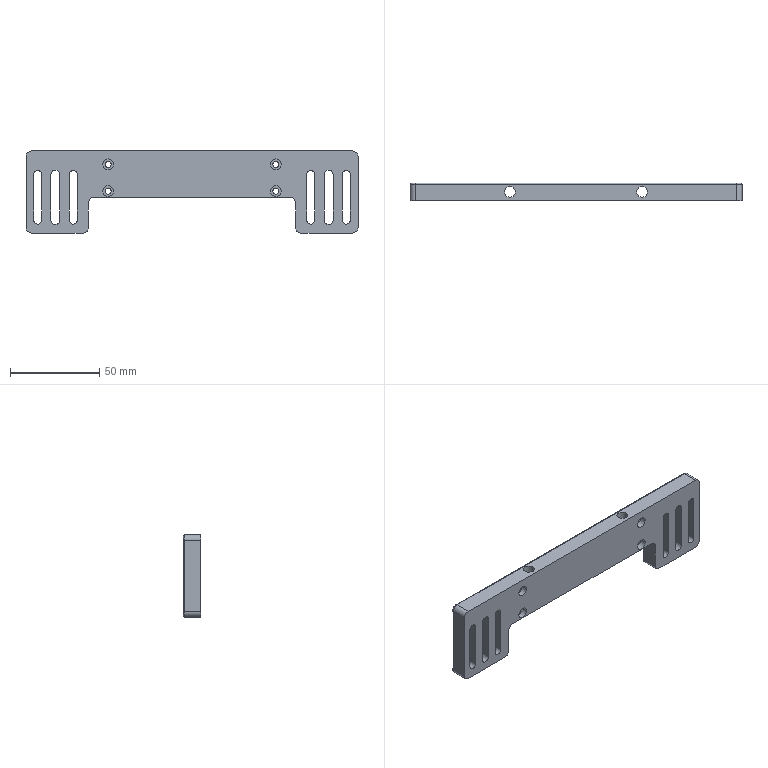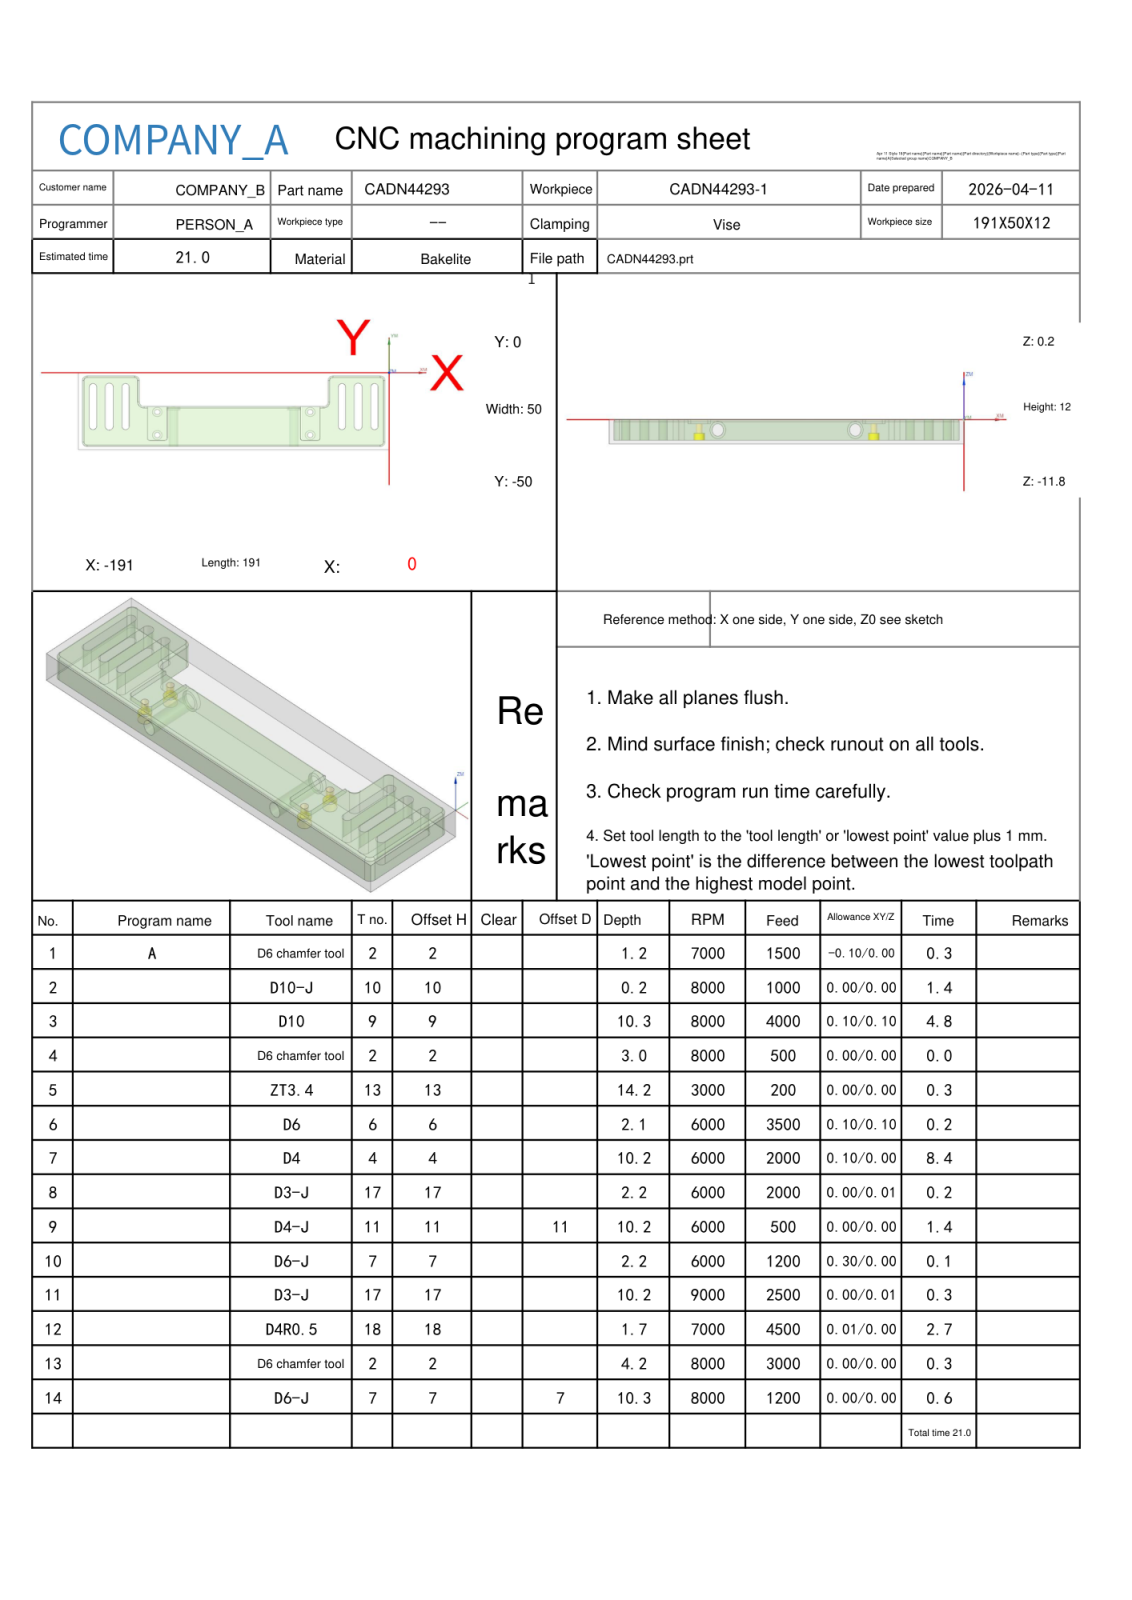NC program | NX | posted by the shop | part box 186 x 10 x 46 mm
Lines 1 to 1587 of 7485:
%
O0001
(Machine time: 23.98 MIN)
(===Total Tool:10===)
(T2=D6 chamfer tool   D=6.   R=0.   D-  H02 Z=-4.   )
(T10=D10-J  D=10.  R=0.   D-  H10 Z=-0.   )
(T9=D10     D=10.  R=0.   D-  H09 Z=-10.1 )
(T13=ZT3.4  D=3.4  DR_a=118 D-  H13 Z=-14.  )
(T6=D6      D=6.   R=0.   D-  H06 Z=-1.9  )
(T4=D4      D=4.   R=0.   D-  H04 Z=-10.  )
(T17=D3-J   D=3.   R=0.   D-  H17 Z=-9.95 )
(T11=D4-J   D=4.   R=0.   D11 H11 Z=-10.  )
(T7=D6-J    D=6.   R=0.   D-  H07 Z=-10.1 )
(T18=D4R0.5 D=4.   R=0.5  D-  H18 Z=-1.5  )
G80 G90 G17 G49 G40
G91 G28 Z0
M01
N1 T02 M06
(D6 chamfer tool  D=6. R=0. H=02 ce=-0.10 di=0.00)
G00 G90 G54 X-152.6 Y-14.634 M03 S7000
G43 H02 Z20.
M08
Z2.5
G01 Y-19.112 Z.87 F1500.
X-152.561 Y-19.417 Z.758
X-152.478 Y-19.714 Z.646
X-152.353 Y-19.995 Z.534
X-152.188 Y-20.254 Z.422
X-151.987 Y-20.487 Z.31
X-151.754 Y-20.688 Z.198
X-151.495 Y-20.853 Z.086
X-151.214 Y-20.978 Z-.025
X-150.917 Y-21.061 Z-.137
X-150.612 Y-21.1 Z-.249
X-148.55 Z-1.
X-40.5
G03 X-38.4 Y-19. I0.0 J2.1
G01 Y-5.
G02 X-34.5 Y-1.1 I3.9 J0.0
G01 X-5.5
G02 X-1.6 Y-5. I0.0 J-3.9
G01 Y-45.
G02 X-5.5 Y-48.9 I-3.9 J0.0
G01 X-185.5
G02 X-189.4 Y-45. I0.0 J3.9
G01 Y-5.
G02 X-185.5 Y-1.1 I3.9 J0.0
G01 X-156.5
G02 X-152.6 Y-5. I0.0 J-3.9
G01 Y-19.
G03 X-150.5 Y-21.1 I2.1 J0.0
G01 X-148.55
X-148.05
Z1.5
G00 Z20.
G91 G28 Z0.0
M05
M09
G91 G28 Z0.0
M01
N2 T10 M06
(D10-J  D=10. R=0. H=10 ce=0.00 di=0.00)
G00 G90 G54 X14.499 Y-44.782 M03 S8000
G43 H10 Z20.
M08
Z2.
G01 Z0.0 F1000.
X2.499 Y-44.912
X-192.413 Y-47.027
X-192.423
G02 X-193.412 Y-46.175 I0.0 J1.
X-193.499 Y-45. I7.912 J1.175
G01 Y-41.202
G02 X-192.511 Y-40.203 I1. J-.001
G01 X1.511 Y-38.098
G03 X2.499 Y-37.099 I-.012 J1.
G01 Y-32.172
G03 X1.599 Y-31.272 I-.9 J0.0
G01 X1.589
X-192.59 Y-33.379
X-192.599
G02 X-193.499 Y-32.48 I0.0 J.9
G01 Y-27.553
G02 X-192.51 Y-26.553 I1. J0.0
G01 X1.511 Y-24.447
G03 X2.499 Y-23.448 I-.012 J1.
G01 Y-18.521
G03 X1.599 Y-17.621 I-.9 J0.0
G01 X1.589
X-192.59 Y-19.728
X-192.599
G02 X-193.499 Y-18.829 I0.0 J.9
G01 Y-13.902
G02 X-192.51 Y-12.902 I1. J0.0
G01 X1.511 Y-10.797
G03 X2.499 Y-9.798 I-.012 J1.
G01 Y-5.
X2.498 Y-4.854
G03 X1.598 Y-3.971 I-.9 J-.017
G01 X1.589
X-193.499 Y-6.088
X-205.499 Y-6.218
Z2.
G00 Z20.
G91 G28 Z0.0
M05
M09
G91 G28 Z0.0
M01
N3 T09 M06
(D10  D=10. R=0. H=09 ce=0.10 di=0.10)
G00 G90 G54 X-62.968 Y12. M03 S8000
G43 H09 Z10.2
M08
Z.719
G01 Z-.481 F4000.
G02 X-61.259 Y7.416 I-5.291 J-4.584
X-61.689 Y5. I-7. J0.0
G03 X-61.821 Y4.634 I27.189 J-10.
G02 X-62.76 Y3.97 I-.942 J.336
G01 X-128.24
G02 X-129.112 Y4.485 I.003 J1.
G03 X-129.986 Y5. I-.874 J-.485
G01 X-135.981
G03 X-136.581 Y4.4 I0.0 J-.6
X-136.526 Y4.15 I.6 J0.0
G02 X-134.714 Y-2.162 I-19.974 J-9.15
G03 X-133.725 Y-3.03 I.991 J.132
G01 X-57.275
G03 X-56.286 Y-2.162 I-.002 J1.
G02 X-54.343 Y4.429 I21.786 J-2.838
X-53.441 Y5. I.903 J-.429
G01 X-46.503
G02 X-46.103 Y4.6 I0.0 J-.4
X-46.191 Y4.35 I-.4 J0.0
G03 X-49.47 Y-5. I11.691 J-9.35
G01 Y-9.685
G02 X-50.47 Y-10.684 I-1. J.001
X-50.78 Y-10.634 I0.0 J1.
G03 X-54.545 Y-10.03 I-3.777 J-11.503
G01 X-136.483
G03 X-140.217 Y-10.645 I.082 J-12.149
G02 X-140.53 Y-10.695 I-.313 J.95
X-141.53 Y-9.696 I0.0 J1.
G01 Y-5.
G03 X-144.743 Y4.267 I-14.97 J0.0
X-145.45 Y4.61 I-.707 J-.557
X-146.051 Y4.38 I0.0 J-.9
G01 X-149.867 Y.954
G03 X-150.199 Y.21 I.668 J-.744
X-150.013 Y-.37 I1. J0.0
G02 X-148.53 Y-5. I-6.487 J-4.63
G01 Y-17.035
G02 X-143.45 Y-22.148 I-.033 J-5.113
G01 Y-22.186
Y-38.9
X-141.55
Y-22.227
Y-22.179
G02 X-136.45 Y-17.03 I5.149 J0.0
G01 X-54.55
G02 X-49.45 Y-22.137 I-.007 J-5.107
G01 Y-22.144
Y-38.9
X-47.55
Y-22.144
G02 X-42.47 Y-17.034 I5.116 J-.006
G01 Y-5.
G02 X-34.5 Y2.97 I7.97 J0.0
G01 X-5.5
G02 X2.47 Y-5. I0.0 J-7.97
G01 Y-45.
G02 X-5.5 Y-52.97 I-7.97 J0.0
G01 X-185.5
G02 X-193.47 Y-45. I0.0 J7.97
G01 Y-5.
G02 X-185.5 Y2.97 I7.97 J0.0
G01 X-156.5
G02 X-148.573 Y-4.171 I0.0 J-7.97
X-148.537 Y-4.67 I-7.927 J-.829
G03 X-141.543 Y-11.38 I6.994 J.29
X-141.253 Y-11.374 I0.0 J7.
G01 Z.719
G00 Z3.
G01 X-63.12 Y12. F6000.
G00 Z.238
G01 Z-.962 F4000.
G02 X-61.401 Y7.406 I-5.281 J-4.594
X-61.827 Y5. I-7. J0.0
G03 X-61.914 Y4.761 I27.327 J-10.
G02 X-62.851 Y4.099 I-.941 J.339
G01 X-128.149
G02 X-128.981 Y4.55 I.004 J1.
G03 X-129.816 Y5. I-.835 J-.55
G01 X-135.839
G03 X-136.438 Y4.4 I0.0 J-.6
X-136.385 Y4.152 I.6 J0.0
G02 X-134.6 Y-2.038 I-20.115 J-9.152
G03 X-133.612 Y-2.901 I.991 J.137
G01 X-57.388
G03 X-56.4 Y-2.038 I-.003 J1.
G02 X-54.488 Y4.427 I21.9 J-2.962
X-53.584 Y5. I.904 J-.427
G01 X-46.668
G02 X-46.268 Y4.6 I0.0 J-.4
X-46.354 Y4.352 I-.4 J0.0
G03 X-49.599 Y-5. I11.854 J-9.352
G01 Y-9.513
G02 X-50.599 Y-10.511 I-1. J.002
X-50.899 Y-10.465 I0.0 J1.
G03 X-54.549 Y-9.901 I-3.652 J-11.537
G01 X-136.451
G03 X-140.101 Y-10.465 I.002 J-12.101
G02 X-140.401 Y-10.511 I-.3 J.954
X-141.401 Y-9.513 I0.0 J1.
G01 Y-5.
G03 X-144.576 Y4.263 I-15.099 J0.0
X-145.286 Y4.611 I-.711 J-.552
X-145.882 Y4.385 I0.0 J-.9
G01 X-149.724 Y.99
G03 X-150.061 Y.241 I.663 J-.749
X-149.879 Y-.335 I1. J0.0
G02 X-148.401 Y-5. I-6.621 J-4.665
G01 Y-16.903
G02 X-143.447 Y-22.008 I-.154 J-5.106
G01 X-143.45 Y-22.186
Y-38.9
X-141.55
Y-22.002
G02 X-136.45 Y-16.901 I5.101 J0.0
G01 X-54.55
G02 X-49.45 Y-22.001 I-.001 J-5.101
G01 Y-38.9
X-47.55
Y-22.002
G02 X-42.599 Y-16.904 I5.102 J-.001
G01 Y-5.
G02 X-34.5 Y3.099 I8.099 J0.0
G01 X-5.5
G02 X2.599 Y-5. I0.0 J-8.099
G01 Y-45.
G02 X-5.5 Y-53.099 I-8.099 J0.0
G01 X-185.5
G02 X-193.599 Y-45. I0.0 J8.099
G01 Y-5.
G02 X-185.5 Y3.099 I8.099 J0.0
G01 X-156.5
G02 X-148.447 Y-4.139 I0.0 J-8.099
X-148.409 Y-4.637 I-8.053 J-.861
G03 X-141.416 Y-11.324 I6.993 J.313
X-141.102 Y-11.317 I0.0 J7.
G01 Z.238
G00 Z2.519
G01 X-63.12 Y12. F6000.
G00 Z-.243
G01 Z-1.443 F4000.
G02 X-61.402 Y7.405 I-5.281 J-4.595
X-61.828 Y5. I-7. J0.0
G03 X-61.914 Y4.761 I27.328 J-10.
G02 X-62.851 Y4.1 I-.941 J.339
G01 X-128.149
G02 X-128.981 Y4.55 I.004 J1.
G03 X-129.815 Y5. I-.835 J-.55
G01 X-135.838
G03 X-136.438 Y4.4 I0.0 J-.6
X-136.384 Y4.152 I.6 J0.0
G02 X-134.599 Y-2.038 I-20.116 J-9.152
G03 X-133.612 Y-2.901 I.991 J.137
G01 X-131.103 Y-2.9
X-59.857 Y-2.901
X-57.388
G03 X-56.401 Y-2.038 I-.003 J1.
G02 X-54.489 Y4.427 I21.901 J-2.962
X-53.585 Y5. I.904 J-.427
G01 X-46.669
G02 X-46.269 Y4.6 I0.0 J-.4
X-46.355 Y4.352 I-.4 J0.0
G03 X-49.6 Y-5. I11.855 J-9.352
G01 Y-9.512
G02 X-50.6 Y-10.51 I-1. J.002
X-50.899 Y-10.464 I0.0 J1.
G03 X-54.55 Y-9.9 I-3.651 J-11.536
G01 X-57.054
X-57.202 Y-9.901
X-57.388
X-59.96 Y-9.9
X-131.072 Y-9.901
X-133.798
X-133.946 Y-9.9
X-136.476
G03 X-140.101 Y-10.464 I.026 J-12.1
G02 X-140.4 Y-10.51 I-.299 J.954
X-141.4 Y-9.512 I0.0 J1.
G01 Y-5.
G03 X-144.575 Y4.263 I-15.1 J0.0
X-145.286 Y4.611 I-.711 J-.552
X-145.881 Y4.385 I0.0 J-.9
G01 X-149.723 Y.99
G03 X-150.061 Y.241 I.663 J-.749
X-149.878 Y-.335 I1. J0.0
G02 X-148.4 Y-5. I-6.622 J-4.665
G01 Y-16.902
G02 X-143.45 Y-22. I-.15 J-5.098
G01 Y-38.9
X-141.55
Y-22.
G02 X-136.45 Y-16.9 I5.1 J0.0
G01 X-133.962
X-133.814 Y-16.901
X-130.971 Y-16.9
X-59.996 Y-16.901
X-57.186
X-57.038 Y-16.9
X-54.55
G02 X-49.45 Y-22. I0.0 J-5.1
G01 Y-38.9
X-47.55
Y-22.
G02 X-42.6 Y-16.902 I5.1 J0.0
G01 Y-5.
G02 X-34.5 Y3.1 I8.1 J0.0
G01 X-5.5
G02 X2.6 Y-5. I0.0 J-8.1
G01 Y-45.
G02 X-5.5 Y-53.1 I-8.1 J0.0
G01 X-185.5
G02 X-193.6 Y-45. I0.0 J8.1
G01 Y-5.
G02 X-185.5 Y3.1 I8.1 J0.0
G01 X-156.5
G02 X-148.446 Y-4.139 I0.0 J-8.1
X-148.408 Y-4.637 I-8.054 J-.861
G03 X-141.415 Y-11.324 I6.993 J.314
X-141.102 Y-11.317 I0.0 J7.
G01 Z-.243
G00 Z2.038
G01 X-63.12 Y12. F6000.
G00 Z-.724
G01 Z-1.924 F4000.
G02 X-61.402 Y7.406 I-5.281 J-4.594
X-61.828 Y5. I-7. J0.0
G03 X-61.914 Y4.761 I27.328 J-10.
G02 X-62.851 Y4.1 I-.941 J.339
G01 X-128.149
G02 X-128.981 Y4.55 I.004 J1.
G03 X-129.815 Y5. I-.835 J-.55
G01 X-135.838
G03 X-136.438 Y4.4 I0.0 J-.6
X-136.384 Y4.152 I.6 J0.0
G02 X-134.599 Y-2.038 I-20.116 J-9.152
G03 X-133.612 Y-2.901 I.991 J.137
G01 X-131.097 Y-2.9
X-59.861 Y-2.901
X-57.388
G03 X-56.401 Y-2.038 I-.003 J1.
G02 X-54.489 Y4.427 I21.901 J-2.962
X-53.585 Y5. I.904 J-.427
G01 X-46.669
G02 X-46.269 Y4.6 I0.0 J-.4
X-46.355 Y4.352 I-.4 J0.0
G03 X-49.6 Y-5. I11.855 J-9.352
G01 Y-8.938
G02 X-50.597 Y-9.935 I-1. J.003
G01 X-53.627
G03 X-54.55 Y-9.9 I-.923 J-12.065
G01 X-57.053
X-57.211 Y-9.901
X-57.388
X-59.963 Y-9.9
X-131.07 Y-9.901
X-133.789
X-133.947 Y-9.9
X-136.761
X-136.869 Y-9.907
G03 X-137.373 Y-9.935 I.419 J-12.093
G01 X-140.403
G02 X-141.4 Y-8.938 I.003 J1.
G01 Y-5.
G03 X-144.575 Y4.263 I-15.1 J0.0
X-145.286 Y4.611 I-.711 J-.552
X-145.881 Y4.385 I0.0 J-.9
G01 X-149.723 Y.99
G03 X-150.061 Y.241 I.663 J-.749
X-149.878 Y-.335 I1. J0.0
G02 X-148.4 Y-5. I-6.622 J-4.665
G01 Y-16.902
G02 X-147.952 Y-16.935 I-.15 J-5.098
G01 X-137.048
G02 X-136.526 Y-16.9 I.604 J-5.065
G01 X-133.962
X-133.803 Y-16.901
X-130.971 Y-16.9
X-59.995 Y-16.901
X-57.197
X-57.038 Y-16.9
X-54.55
G02 X-53.952 Y-16.935 I0.0 J-5.1
G01 X-43.048
G02 X-42.6 Y-16.902 I.598 J-5.065
G01 Y-5.
G02 X-34.5 Y3.1 I8.1 J0.0
G01 X-5.5
G02 X2.6 Y-5. I0.0 J-8.1
G01 Y-45.
G02 X-5.5 Y-53.1 I-8.1 J0.0
G01 X-185.5
G02 X-193.6 Y-45. I0.0 J8.1
G01 Y-5.
G02 X-185.5 Y3.1 I8.1 J0.0
G01 X-156.5
G02 X-148.446 Y-4.139 I0.0 J-8.1
X-148.408 Y-4.637 I-8.054 J-.861
G03 X-141.415 Y-11.324 I6.993 J.314
X-141.102 Y-11.317 I0.0 J7.
G01 Z-.724
G00 Z1.557
G01 X-63.12 Y12. F6000.
G00 Z-1.205
G01 Z-2.405 F4000.
G02 X-61.402 Y7.405 I-5.281 J-4.595
X-61.828 Y5. I-7. J0.0
G03 X-61.914 Y4.76 I27.328 J-10.
G02 X-62.851 Y4.1 I-.941 J.34
G01 X-128.149
G02 X-128.981 Y4.55 I.004 J1.
G03 X-129.815 Y5. I-.835 J-.55
G01 X-135.838
G03 X-136.438 Y4.4 I0.0 J-.6
X-136.384 Y4.152 I.6 J0.0
G02 X-134.599 Y-2.038 I-20.116 J-9.152
G03 X-133.613 Y-2.901 I.99 J.138
G01 X-131.092 Y-2.9
X-59.861 Y-2.901
X-57.387
G03 X-56.401 Y-2.038 I-.004 J1.
G02 X-54.489 Y4.427 I21.901 J-2.962
X-53.585 Y5. I.904 J-.427
G01 X-46.669
G02 X-46.269 Y4.6 I0.0 J-.4
X-46.355 Y4.352 I-.4 J0.0
G03 X-49.6 Y-5. I11.855 J-9.352
G01 Y-8.903
G02 X-50.597 Y-9.9 I-1. J.003
G01 X-57.052
X-57.222 Y-9.901
X-57.387
X-59.963 Y-9.9
X-131.069 Y-9.901
X-133.778
X-133.948 Y-9.9
X-140.403
G02 X-141.4 Y-8.903 I.003 J1.
G01 Y-5.
G03 X-144.575 Y4.263 I-15.1 J0.0
X-145.286 Y4.611 I-.711 J-.552
X-145.881 Y4.385 I0.0 J-.9
G01 X-149.723 Y.99
G03 X-150.061 Y.241 I.663 J-.749
X-149.878 Y-.335 I1. J0.0
G02 X-148.4 Y-5. I-6.622 J-4.665
G01 Y-16.9
X-133.962
X-133.792 Y-16.901
X-130.971 Y-16.9
X-59.995 Y-16.901
X-57.208
X-57.038 Y-16.9
X-42.6
Y-5.
G02 X-34.5 Y3.1 I8.1 J0.0
G01 X-5.5
G02 X2.6 Y-5. I0.0 J-8.1
G01 Y-45.
G02 X-5.5 Y-53.1 I-8.1 J0.0
G01 X-185.5
G02 X-193.6 Y-45. I0.0 J8.1
G01 Y-5.
G02 X-185.5 Y3.1 I8.1 J0.0
G01 X-156.5
G02 X-148.446 Y-4.139 I0.0 J-8.1
X-148.408 Y-4.637 I-8.054 J-.861
G03 X-141.415 Y-11.324 I6.993 J.314
X-141.102 Y-11.317 I0.0 J7.
G01 Z-1.205
G00 Z1.076
G01 X-63.12 Y12. F6000.
G00 Z-1.686
G01 Z-2.886 F4000.
G02 X-61.402 Y7.406 I-5.281 J-4.595
X-61.828 Y5. I-7. J0.0
G03 X-61.914 Y4.76 I27.328 J-10.
G02 X-62.85 Y4.1 I-.941 J.34
G01 X-128.15
G02 X-128.981 Y4.55 I.004 J1.
G03 X-129.815 Y5. I-.835 J-.55
G01 X-135.838
G03 X-136.438 Y4.4 I0.0 J-.6
X-136.384 Y4.152 I.6 J0.0
G02 X-134.599 Y-2.039 I-20.116 J-9.152
G03 X-133.613 Y-2.901 I.99 J.138
G01 X-131.086 Y-2.9
X-59.865 Y-2.901
X-57.387
G03 X-56.401 Y-2.039 I-.004 J1.
G02 X-54.489 Y4.427 I21.901 J-2.961
X-53.585 Y5. I.904 J-.427
G01 X-46.669
G02 X-46.269 Y4.6 I0.0 J-.4
X-46.355 Y4.352 I-.4 J0.0
G03 X-49.6 Y-5. I11.855 J-9.352
G01 Y-8.903
G02 X-50.597 Y-9.9 I-1. J.003
G01 X-57.051
X-57.234 Y-9.901
X-57.387
X-59.965 Y-9.9
X-131.068 Y-9.901
X-133.766
X-133.949 Y-9.9
X-140.403
G02 X-141.4 Y-8.903 I.003 J1.
G01 Y-5.
G03 X-144.575 Y4.263 I-15.1 J0.0
X-145.286 Y4.611 I-.711 J-.552
X-145.881 Y4.385 I0.0 J-.9
G01 X-149.723 Y.99
G03 X-150.061 Y.241 I.663 J-.749
X-149.878 Y-.335 I1. J0.0
G02 X-148.4 Y-5. I-6.622 J-4.665
G01 Y-16.9
X-133.962
X-133.779 Y-16.901
X-130.971 Y-16.9
X-59.993 Y-16.901
X-57.221
X-57.038 Y-16.9
X-42.6
Y-5.
G02 X-34.5 Y3.1 I8.1 J0.0
G01 X-5.5
G02 X2.6 Y-5. I0.0 J-8.1
G01 Y-45.
G02 X-5.5 Y-53.1 I-8.1 J0.0
G01 X-185.5
G02 X-193.6 Y-45. I0.0 J8.1
G01 Y-5.
G02 X-185.5 Y3.1 I8.1 J0.0
G01 X-156.5
G02 X-148.446 Y-4.139 I0.0 J-8.1
X-148.408 Y-4.637 I-8.054 J-.861
G03 X-141.415 Y-11.324 I6.993 J.314
X-141.102 Y-11.317 I0.0 J7.
G01 Z-1.686
G00 Z.595
G01 X-63.12 Y12. F6000.
G00 Z-2.167
G01 Z-3.367 F4000.
G02 X-61.402 Y7.406 I-5.281 J-4.594
X-61.828 Y5. I-7. J0.0
G03 X-61.914 Y4.76 I27.328 J-10.
G02 X-62.85 Y4.1 I-.94 J.34
G01 X-128.15
G02 X-128.981 Y4.55 I.005 J1.
G03 X-129.815 Y5. I-.835 J-.55
G01 X-135.838
G03 X-136.438 Y4.4 I0.0 J-.6
X-136.384 Y4.152 I.6 J0.0
G02 X-134.599 Y-2.039 I-20.116 J-9.152
G03 X-133.613 Y-2.901 I.99 J.138
G01 X-131.083 Y-2.9
X-59.865 Y-2.901
X-57.387
G03 X-56.401 Y-2.039 I-.004 J1.
G02 X-54.489 Y4.427 I21.901 J-2.961
X-53.585 Y5. I.904 J-.427
G01 X-46.669
G02 X-46.269 Y4.6 I0.0 J-.4
X-46.355 Y4.352 I-.4 J0.0
G03 X-49.6 Y-5. I11.855 J-9.352
G01 Y-8.904
G02 X-50.596 Y-9.9 I-1. J.004
G01 X-57.05
X-57.249 Y-9.901
X-57.387
X-59.965 Y-9.9
X-131.068 Y-9.901
X-133.751
X-133.95 Y-9.9
X-140.404
G02 X-141.4 Y-8.904 I.004 J1.
G01 Y-5.
G03 X-144.575 Y4.263 I-15.1 J0.0
X-145.286 Y4.611 I-.711 J-.552
X-145.881 Y4.385 I0.0 J-.9
G01 X-149.723 Y.99
G03 X-150.061 Y.241 I.663 J-.749
X-149.878 Y-.335 I1. J0.0
G02 X-148.4 Y-5. I-6.622 J-4.665
G01 Y-16.9
X-133.962
X-133.763 Y-16.901
X-130.971 Y-16.9
X-59.993 Y-16.901
X-57.237
X-57.038 Y-16.9
X-42.6
Y-5.
G02 X-34.5 Y3.1 I8.1 J0.0
G01 X-5.5
G02 X2.6 Y-5. I0.0 J-8.1
G01 Y-45.
G02 X-5.5 Y-53.1 I-8.1 J0.0
G01 X-185.5
G02 X-193.6 Y-45. I0.0 J8.1
G01 Y-5.
G02 X-185.5 Y3.1 I8.1 J0.0
G01 X-156.5
G02 X-148.446 Y-4.139 I0.0 J-8.1
X-148.408 Y-4.637 I-8.054 J-.861
G03 X-141.415 Y-11.324 I6.993 J.314
X-141.102 Y-11.317 I0.0 J7.
G01 Z-2.167
G00 Z.114
G01 X-63.12 Y12. F6000.
G00 Z-2.648
G01 Z-3.848 F4000.
G02 X-61.402 Y7.406 I-5.281 J-4.595
X-61.828 Y5. I-7. J0.0
G03 X-61.914 Y4.76 I27.328 J-10.
G02 X-62.85 Y4.1 I-.94 J.34
G01 X-128.15
G02 X-128.981 Y4.55 I.005 J1.
G03 X-129.815 Y5. I-.835 J-.55
G01 X-135.838
G03 X-136.438 Y4.4 I0.0 J-.6
X-136.384 Y4.152 I.6 J0.0
G02 X-134.599 Y-2.039 I-20.116 J-9.152
G03 X-133.613 Y-2.901 I.99 J.138
G01 X-131.083 Y-2.9
X-59.867 Y-2.901
X-57.387
G03 X-56.401 Y-2.039 I-.004 J1.
G02 X-54.489 Y4.427 I21.901 J-2.961
X-53.585 Y5. I.904 J-.427
G01 X-46.669
G02 X-46.269 Y4.6 I0.0 J-.4
X-46.355 Y4.352 I-.4 J0.0
G03 X-49.6 Y-5. I11.855 J-9.352
G01 Y-8.904
G02 X-50.596 Y-9.9 I-1. J.004
G01 X-57.049
X-57.266 Y-9.901
X-57.387
X-59.967 Y-9.9
X-131.068 Y-9.901
X-133.734
X-133.951 Y-9.9
X-140.404
G02 X-141.4 Y-8.904 I.004 J1.
G01 Y-5.
G03 X-144.575 Y4.263 I-15.1 J0.0
X-145.286 Y4.611 I-.711 J-.552
X-145.881 Y4.385 I0.0 J-.9
G01 X-149.723 Y.99
G03 X-150.061 Y.241 I.663 J-.749
X-149.878 Y-.335 I1. J0.0
G02 X-148.4 Y-5. I-6.622 J-4.665
G01 Y-16.9
X-133.962
X-133.745 Y-16.901
X-130.971 Y-16.9
X-59.992 Y-16.901
X-57.255
X-57.038 Y-16.9
X-42.6
Y-5.
G02 X-34.5 Y3.1 I8.1 J0.0
G01 X-5.5
G02 X2.6 Y-5. I0.0 J-8.1
G01 Y-45.
G02 X-5.5 Y-53.1 I-8.1 J0.0
G01 X-185.5
G02 X-193.6 Y-45. I0.0 J8.1
G01 Y-5.
G02 X-185.5 Y3.1 I8.1 J0.0
G01 X-156.5
G02 X-148.446 Y-4.139 I0.0 J-8.1
X-148.408 Y-4.637 I-8.054 J-.861
G03 X-141.415 Y-11.324 I6.993 J.314
X-141.102 Y-11.317 I0.0 J7.
G01 Z-2.648
G00 Z-.367
G01 X-63.12 Y12. F6000.
G00 Z-3.129
G01 Z-4.329 F4000.
G02 X-61.402 Y7.406 I-5.281 J-4.595
X-61.828 Y5. I-7. J0.0
G03 X-61.914 Y4.762 I27.328 J-10.
G02 X-62.852 Y4.1 I-.941 J.338
G01 X-128.148
G02 X-128.981 Y4.55 I.003 J1.
G03 X-129.815 Y5. I-.835 J-.55
G01 X-135.838
G03 X-136.438 Y4.4 I0.0 J-.6
X-136.384 Y4.152 I.6 J0.0
G02 X-134.6 Y-2.036 I-20.116 J-9.152
G03 X-133.611 Y-2.9 I.991 J.136
G01 X-57.389
G03 X-56.4 Y-2.036 I-.002 J1.
G02 X-54.489 Y4.427 I21.9 J-2.964
X-53.585 Y5. I.904 J-.427
G01 X-46.669
G02 X-46.269 Y4.6 I0.0 J-.4
X-46.355 Y4.352 I-.4 J0.0
G03 X-49.6 Y-5. I11.855 J-9.352
G01 Y-8.901
G02 X-50.599 Y-9.9 I-1. J.001
G01 X-140.401
G02 X-141.4 Y-8.901 I.001 J1.
G01 Y-5.
G03 X-144.575 Y4.263 I-15.1 J0.0
X-145.286 Y4.611 I-.711 J-.552
X-145.881 Y4.385 I0.0 J-.9
G01 X-149.723 Y.99
G03 X-150.061 Y.241 I.663 J-.749
X-149.878 Y-.335 I1. J0.0
G02 X-148.4 Y-5. I-6.622 J-4.665
G01 Y-16.9
X-42.6
Y-5.
G02 X-34.5 Y3.1 I8.1 J0.0
G01 X-5.5
G02 X2.6 Y-5. I0.0 J-8.1
G01 Y-45.
G02 X-5.5 Y-53.1 I-8.1 J0.0
G01 X-185.5
G02 X-193.6 Y-45. I0.0 J8.1
G01 Y-5.
G02 X-185.5 Y3.1 I8.1 J0.0
G01 X-156.5
G02 X-148.446 Y-4.139 I0.0 J-8.1
X-148.408 Y-4.637 I-8.054 J-.861
G03 X-141.415 Y-11.324 I6.993 J.314
X-141.102 Y-11.317 I0.0 J7.
G01 Z-3.129
G00 Z-.848
G01 X-63.12 Y12. F6000.
G00 Z-3.61
G01 Z-4.81 F4000.
G02 X-61.402 Y7.405 I-5.281 J-4.595
X-61.828 Y5. I-7. J0.0
G03 X-61.914 Y4.761 I27.328 J-10.
G02 X-62.852 Y4.1 I-.941 J.339
G01 X-128.148
G02 X-128.981 Y4.55 I.003 J1.
G03 X-129.815 Y5. I-.835 J-.55
G01 X-135.838
G03 X-136.438 Y4.4 I0.0 J-.6
X-136.384 Y4.152 I.6 J0.0
G02 X-134.6 Y-2.037 I-20.116 J-9.152
G03 X-133.611 Y-2.9 I.991 J.137
G01 X-57.389
G03 X-56.4 Y-2.037 I-.002 J1.
G02 X-54.489 Y4.427 I21.9 J-2.963
X-53.585 Y5. I.904 J-.427
G01 X-46.669
G02 X-46.269 Y4.6 I0.0 J-.4
X-46.355 Y4.352 I-.4 J0.0
G03 X-49.6 Y-5. I11.855 J-9.352
G01 Y-8.901
G02 X-50.599 Y-9.9 I-1. J.001
G01 X-140.401
G02 X-141.4 Y-8.901 I.001 J1.
G01 Y-5.
G03 X-144.575 Y4.263 I-15.1 J0.0
X-145.286 Y4.611 I-.711 J-.552
X-145.881 Y4.385 I0.0 J-.9
G01 X-149.723 Y.99
G03 X-150.061 Y.241 I.663 J-.749
X-149.878 Y-.335 I1. J0.0
G02 X-148.4 Y-5. I-6.622 J-4.665
G01 Y-16.9
X-42.6
Y-5.
G02 X-34.5 Y3.1 I8.1 J0.0
G01 X-5.5
G02 X2.6 Y-5. I0.0 J-8.1
G01 Y-45.
G02 X-5.5 Y-53.1 I-8.1 J0.0
G01 X-185.5
G02 X-193.6 Y-45. I0.0 J8.1
G01 Y-5.
G02 X-185.5 Y3.1 I8.1 J0.0
G01 X-156.5
G02 X-148.446 Y-4.139 I0.0 J-8.1
X-148.408 Y-4.637 I-8.054 J-.861
G03 X-141.415 Y-11.324 I6.993 J.314
X-141.102 Y-11.317 I0.0 J7.
G01 Z-3.61
G00 Z-1.329
G01 X-63.12 Y12. F6000.
G00 Z-4.09
G01 Z-5.29 F4000.
G02 X-61.402 Y7.406 I-5.281 J-4.595
X-61.828 Y5. I-7. J0.0
G03 X-61.914 Y4.762 I27.328 J-10.
G02 X-62.852 Y4.1 I-.941 J.338
G01 X-128.148
G02 X-128.981 Y4.55 I.003 J1.
G03 X-129.815 Y5. I-.835 J-.55
G01 X-135.838
G03 X-136.438 Y4.4 I0.0 J-.6
X-136.384 Y4.152 I.6 J0.0
G02 X-134.6 Y-2.036 I-20.116 J-9.152
G03 X-133.611 Y-2.9 I.991 J.136
G01 X-57.389
G03 X-56.4 Y-2.036 I-.002 J1.
G02 X-54.489 Y4.427 I21.9 J-2.964
X-53.585 Y5. I.904 J-.427
G01 X-46.669
G02 X-46.269 Y4.6 I0.0 J-.4
X-46.355 Y4.352 I-.4 J0.0
G03 X-49.6 Y-5. I11.855 J-9.352
G01 Y-8.901
G02 X-50.599 Y-9.9 I-1. J.001
G01 X-140.401
G02 X-141.4 Y-8.901 I.001 J1.
G01 Y-5.
G03 X-144.575 Y4.263 I-15.1 J0.0
X-145.286 Y4.611 I-.711 J-.552
X-145.881 Y4.385 I0.0 J-.9
G01 X-149.723 Y.99
G03 X-150.061 Y.241 I.663 J-.749
X-149.878 Y-.335 I1. J0.0
G02 X-148.4 Y-5. I-6.622 J-4.665
G01 Y-16.9
X-42.6
Y-5.
G02 X-34.5 Y3.1 I8.1 J0.0
G01 X-5.5
G02 X2.6 Y-5. I0.0 J-8.1
G01 Y-45.
G02 X-5.5 Y-53.1 I-8.1 J0.0
G01 X-185.5
G02 X-193.6 Y-45. I0.0 J8.1
G01 Y-5.
G02 X-185.5 Y3.1 I8.1 J0.0
G01 X-156.5
G02 X-148.446 Y-4.139 I0.0 J-8.1
X-148.408 Y-4.637 I-8.054 J-.861
G03 X-141.415 Y-11.324 I6.993 J.314
X-141.102 Y-11.317 I0.0 J7.
G01 Z-4.09
G00 Z-1.81
G01 X-63.12 Y12. F6000.
G00 Z-4.571
G01 Z-5.771 F4000.
G02 X-61.402 Y7.405 I-5.281 J-4.595
X-61.828 Y5. I-7. J0.0
G03 X-61.914 Y4.761 I27.328 J-10.
G02 X-62.852 Y4.1 I-.941 J.339
G01 X-128.148
G02 X-128.981 Y4.55 I.003 J1.
G03 X-129.815 Y5. I-.835 J-.55
G01 X-135.838
G03 X-136.438 Y4.4 I0.0 J-.6
X-136.384 Y4.152 I.6 J0.0
G02 X-134.6 Y-2.037 I-20.116 J-9.152
G03 X-133.611 Y-2.9 I.991 J.137
G01 X-57.389
G03 X-56.4 Y-2.037 I-.002 J1.
G02 X-54.489 Y4.427 I21.9 J-2.963
X-53.585 Y5. I.904 J-.427
G01 X-46.669
G02 X-46.269 Y4.6 I0.0 J-.4
X-46.355 Y4.352 I-.4 J0.0
G03 X-49.6 Y-5. I11.855 J-9.352
G01 Y-8.901
G02 X-50.599 Y-9.9 I-1. J.001
G01 X-140.401
G02 X-141.4 Y-8.901 I.001 J1.
G01 Y-5.
G03 X-144.575 Y4.263 I-15.1 J0.0
X-145.286 Y4.611 I-.711 J-.552
X-145.881 Y4.385 I0.0 J-.9
G01 X-149.723 Y.99
G03 X-150.061 Y.241 I.663 J-.749
X-149.878 Y-.335 I1. J0.0
G02 X-148.4 Y-5. I-6.622 J-4.665
G01 Y-16.9
X-42.6
Y-5.
G02 X-34.5 Y3.1 I8.1 J0.0
G01 X-5.5
G02 X2.6 Y-5. I0.0 J-8.1
G01 Y-45.
G02 X-5.5 Y-53.1 I-8.1 J0.0
G01 X-185.5
G02 X-193.6 Y-45. I0.0 J8.1
G01 Y-5.
G02 X-185.5 Y3.1 I8.1 J0.0
G01 X-156.5
G02 X-148.446 Y-4.139 I0.0 J-8.1
X-148.408 Y-4.637 I-8.054 J-.861
G03 X-141.415 Y-11.324 I6.993 J.314
X-141.102 Y-11.317 I0.0 J7.
G01 Z-4.571
G00 Z-2.29
G01 X-63.12 Y12. F6000.
G00 Z-5.052
G01 Z-6.252 F4000.
G02 X-61.402 Y7.406 I-5.281 J-4.595
X-61.828 Y5. I-7. J0.0
G03 X-61.914 Y4.762 I27.328 J-10.
G02 X-62.852 Y4.1 I-.941 J.338
G01 X-128.148
G02 X-128.981 Y4.55 I.003 J1.
G03 X-129.815 Y5. I-.835 J-.55
G01 X-135.838
G03 X-136.438 Y4.4 I0.0 J-.6
X-136.384 Y4.152 I.6 J0.0
G02 X-134.6 Y-2.036 I-20.116 J-9.152
G03 X-133.611 Y-2.9 I.991 J.136
G01 X-57.389
G03 X-56.4 Y-2.036 I-.002 J1.
G02 X-54.489 Y4.427 I21.9 J-2.964
X-53.585 Y5. I.904 J-.427
G01 X-46.669
G02 X-46.269 Y4.6 I0.0 J-.4
X-46.355 Y4.352 I-.4 J0.0
G03 X-49.6 Y-5. I11.855 J-9.352
G01 Y-8.901
G02 X-50.599 Y-9.9 I-1. J.001
G01 X-140.401
G02 X-141.4 Y-8.901 I.001 J1.
G01 Y-5.
G03 X-144.575 Y4.263 I-15.1 J0.0
X-145.286 Y4.611 I-.711 J-.552
X-145.881 Y4.385 I0.0 J-.9
G01 X-149.723 Y.99
G03 X-150.061 Y.241 I.663 J-.749
X-149.878 Y-.335 I1. J0.0
G02 X-148.4 Y-5. I-6.622 J-4.665
G01 Y-16.9
X-42.6
Y-5.
G02 X-34.5 Y3.1 I8.1 J0.0
G01 X-5.5
G02 X2.6 Y-5. I0.0 J-8.1
G01 Y-45.
G02 X-5.5 Y-53.1 I-8.1 J0.0
G01 X-185.5
G02 X-193.6 Y-45. I0.0 J8.1
G01 Y-5.
G02 X-185.5 Y3.1 I8.1 J0.0
G01 X-156.5
G02 X-148.446 Y-4.139 I0.0 J-8.1
X-148.408 Y-4.637 I-8.054 J-.861
G03 X-141.415 Y-11.324 I6.993 J.314
X-141.102 Y-11.317 I0.0 J7.
G01 Z-5.052
G00 Z-2.771
G01 X-63.12 Y12. F6000.
G00 Z-5.533
G01 Z-6.733 F4000.
G02 X-61.402 Y7.405 I-5.281 J-4.595
X-61.828 Y5. I-7. J0.0
G03 X-61.914 Y4.761 I27.328 J-10.
G02 X-62.852 Y4.1 I-.941 J.339
G01 X-128.148
G02 X-128.981 Y4.55 I.003 J1.
G03 X-129.815 Y5. I-.835 J-.55
G01 X-135.838
G03 X-136.438 Y4.4 I0.0 J-.6
X-136.384 Y4.152 I.6 J0.0
G02 X-134.6 Y-2.037 I-20.116 J-9.152
G03 X-133.611 Y-2.9 I.991 J.137
G01 X-57.389
G03 X-56.4 Y-2.037 I-.002 J1.
G02 X-54.489 Y4.427 I21.9 J-2.963
X-53.585 Y5. I.904 J-.427
G01 X-46.669
G02 X-46.269 Y4.6 I0.0 J-.4
X-46.355 Y4.352 I-.4 J0.0
G03 X-49.6 Y-5. I11.855 J-9.352
G01 Y-8.901
G02 X-50.599 Y-9.9 I-1. J.001
G01 X-140.401
G02 X-141.4 Y-8.901 I.001 J1.
G01 Y-5.
G03 X-144.575 Y4.263 I-15.1 J0.0
X-145.286 Y4.611 I-.711 J-.552
X-145.881 Y4.385 I0.0 J-.9
G01 X-149.723 Y.99
G03 X-150.061 Y.241 I.663 J-.749
X-149.878 Y-.335 I1. J0.0
G02 X-148.4 Y-5. I-6.622 J-4.665
G01 Y-16.9
X-42.6
Y-5.
G02 X-34.5 Y3.1 I8.1 J0.0
G01 X-5.5
G02 X2.6 Y-5. I0.0 J-8.1
G01 Y-45.
G02 X-5.5 Y-53.1 I-8.1 J0.0
G01 X-185.5
G02 X-193.6 Y-45. I0.0 J8.1
G01 Y-5.
G02 X-185.5 Y3.1 I8.1 J0.0
G01 X-156.5
G02 X-148.446 Y-4.139 I0.0 J-8.1
X-148.408 Y-4.637 I-8.054 J-.861
G03 X-141.415 Y-11.324 I6.993 J.314
X-141.102 Y-11.317 I0.0 J7.
G01 Z-5.533
G00 Z-3.252
G01 X-63.12 Y12. F6000.
G00 Z-6.014
G01 Z-7.214 F4000.
G02 X-61.402 Y7.406 I-5.281 J-4.595
X-61.828 Y5. I-7. J0.0
G03 X-61.914 Y4.762 I27.328 J-10.
G02 X-62.852 Y4.1 I-.941 J.338
G01 X-128.148
G02 X-128.981 Y4.55 I.003 J1.
G03 X-129.815 Y5. I-.835 J-.55
G01 X-135.838
G03 X-136.438 Y4.4 I0.0 J-.6
X-136.384 Y4.152 I.6 J0.0
G02 X-134.6 Y-2.036 I-20.116 J-9.152
G03 X-133.611 Y-2.9 I.991 J.136
G01 X-57.389
G03 X-56.4 Y-2.036 I-.002 J1.
G02 X-54.489 Y4.427 I21.9 J-2.964
X-53.585 Y5. I.904 J-.427
G01 X-46.669
G02 X-46.269 Y4.6 I0.0 J-.4
X-46.355 Y4.352 I-.4 J0.0
G03 X-49.6 Y-5. I11.855 J-9.352
G01 Y-8.901
G02 X-50.599 Y-9.9 I-1. J.001
G01 X-140.401
G02 X-141.4 Y-8.901 I.001 J1.
G01 Y-5.
G03 X-144.575 Y4.263 I-15.1 J0.0
X-145.286 Y4.611 I-.711 J-.552
X-145.881 Y4.385 I0.0 J-.9
G01 X-149.723 Y.99
G03 X-150.061 Y.241 I.663 J-.749
X-149.878 Y-.335 I1. J0.0
G02 X-148.4 Y-5. I-6.622 J-4.665
G01 Y-16.9
X-42.6
Y-5.
G02 X-34.5 Y3.1 I8.1 J0.0
G01 X-5.5
G02 X2.6 Y-5. I0.0 J-8.1
G01 Y-45.
G02 X-5.5 Y-53.1 I-8.1 J0.0
G01 X-185.5
G02 X-193.6 Y-45. I0.0 J8.1
G01 Y-5.
G02 X-185.5 Y3.1 I8.1 J0.0
G01 X-156.5
G02 X-148.446 Y-4.139 I0.0 J-8.1
X-148.408 Y-4.637 I-8.054 J-.861
G03 X-141.415 Y-11.324 I6.993 J.314
X-141.102 Y-11.317 I0.0 J7.
G01 Z-6.014
G00 Z-3.733
G01 X-63.12 Y12. F6000.
G00 Z-6.495
G01 Z-7.695 F4000.
G02 X-61.402 Y7.405 I-5.281 J-4.595
X-61.828 Y5. I-7. J0.0
G03 X-61.914 Y4.761 I27.328 J-10.
G02 X-62.852 Y4.1 I-.941 J.339
G01 X-128.148
G02 X-128.981 Y4.55 I.003 J1.
G03 X-129.815 Y5. I-.835 J-.55
G01 X-135.838
G03 X-136.438 Y4.4 I0.0 J-.6
X-136.384 Y4.152 I.6 J0.0
G02 X-134.6 Y-2.037 I-20.116 J-9.152
G03 X-133.611 Y-2.9 I.991 J.137
G01 X-57.389
G03 X-56.4 Y-2.037 I-.002 J1.
G02 X-54.489 Y4.427 I21.9 J-2.963
X-53.585 Y5. I.904 J-.427
G01 X-46.669
G02 X-46.269 Y4.6 I0.0 J-.4
X-46.355 Y4.352 I-.4 J0.0
G03 X-49.6 Y-5. I11.855 J-9.352
G01 Y-8.901
G02 X-50.599 Y-9.9 I-1. J.001
G01 X-140.401
G02 X-141.4 Y-8.901 I.001 J1.
G01 Y-5.
G03 X-144.575 Y4.263 I-15.1 J0.0
X-145.286 Y4.611 I-.711 J-.552
X-145.881 Y4.385 I0.0 J-.9
G01 X-149.723 Y.99
G03 X-150.061 Y.241 I.663 J-.749
X-149.878 Y-.335 I1. J0.0
G02 X-148.4 Y-5. I-6.622 J-4.665
G01 Y-16.9
X-42.6
Y-5.
G02 X-34.5 Y3.1 I8.1 J0.0
G01 X-5.5
G02 X2.6 Y-5. I0.0 J-8.1
G01 Y-45.
G02 X-5.5 Y-53.1 I-8.1 J0.0
G01 X-185.5
G02 X-193.6 Y-45. I0.0 J8.1
G01 Y-5.
G02 X-185.5 Y3.1 I8.1 J0.0
G01 X-156.5
G02 X-148.446 Y-4.139 I0.0 J-8.1
X-148.408 Y-4.637 I-8.054 J-.861
G03 X-141.415 Y-11.324 I6.993 J.314
X-141.102 Y-11.317 I0.0 J7.
G01 Z-6.495
G00 Z-4.214
G01 X-63.12 Y12. F6000.
G00 Z-6.976
G01 Z-8.176 F4000.
G02 X-61.402 Y7.406 I-5.281 J-4.595
X-61.828 Y5. I-7. J0.0
G03 X-61.914 Y4.762 I27.328 J-10.
G02 X-62.852 Y4.1 I-.941 J.338
G01 X-128.148
G02 X-128.981 Y4.55 I.003 J1.
G03 X-129.815 Y5. I-.835 J-.55
G01 X-135.838
G03 X-136.438 Y4.4 I0.0 J-.6
X-136.384 Y4.152 I.6 J0.0
G02 X-134.6 Y-2.036 I-20.116 J-9.152
G03 X-133.611 Y-2.9 I.991 J.136
G01 X-57.389
G03 X-56.4 Y-2.036 I-.002 J1.
G02 X-54.489 Y4.427 I21.9 J-2.964
X-53.585 Y5. I.904 J-.427
G01 X-46.669
G02 X-46.269 Y4.6 I0.0 J-.4
X-46.355 Y4.352 I-.4 J0.0
G03 X-49.6 Y-5. I11.855 J-9.352
G01 Y-8.901
G02 X-50.599 Y-9.9 I-1. J.001
G01 X-140.401
G02 X-141.4 Y-8.901 I.001 J1.
G01 Y-5.
G03 X-144.575 Y4.263 I-15.1 J0.0
X-145.286 Y4.611 I-.711 J-.552
X-145.881 Y4.385 I0.0 J-.9
G01 X-149.723 Y.99
G03 X-150.061 Y.241 I.663 J-.749
X-149.878 Y-.335 I1. J0.0
G02 X-148.4 Y-5. I-6.622 J-4.665
G01 Y-16.9
X-42.6
Y-5.
G02 X-34.5 Y3.1 I8.1 J0.0
G01 X-5.5
G02 X2.6 Y-5. I0.0 J-8.1
G01 Y-45.
G02 X-5.5 Y-53.1 I-8.1 J0.0
G01 X-185.5
G02 X-193.6 Y-45. I0.0 J8.1
G01 Y-5.
G02 X-185.5 Y3.1 I8.1 J0.0
G01 X-156.5
G02 X-148.446 Y-4.139 I0.0 J-8.1
X-148.408 Y-4.637 I-8.054 J-.861
G03 X-141.415 Y-11.324 I6.993 J.314
X-141.102 Y-11.317 I0.0 J7.
G01 Z-6.976
G00 Z-4.695
G01 X-63.12 Y12. F6000.
G00 Z-7.457
G01 Z-8.657 F4000.
G02 X-61.402 Y7.405 I-5.281 J-4.595
X-61.828 Y5. I-7. J0.0
G03 X-61.914 Y4.761 I27.328 J-10.
G02 X-62.852 Y4.1 I-.941 J.339
G01 X-128.148
G02 X-128.981 Y4.55 I.003 J1.
G03 X-129.815 Y5. I-.835 J-.55
G01 X-135.838
G03 X-136.438 Y4.4 I0.0 J-.6
X-136.384 Y4.152 I.6 J0.0
G02 X-134.6 Y-2.037 I-20.116 J-9.152
G03 X-133.611 Y-2.9 I.991 J.137
G01 X-57.389
G03 X-56.4 Y-2.037 I-.002 J1.
G02 X-54.489 Y4.427 I21.9 J-2.963
X-53.585 Y5. I.904 J-.427
G01 X-46.669
G02 X-46.269 Y4.6 I0.0 J-.4
X-46.355 Y4.352 I-.4 J0.0
G03 X-49.6 Y-5. I11.855 J-9.352
G01 Y-8.901
G02 X-50.599 Y-9.9 I-1. J.001
G01 X-140.401
G02 X-141.4 Y-8.901 I.001 J1.
G01 Y-5.
G03 X-144.575 Y4.263 I-15.1 J0.0
X-145.286 Y4.611 I-.711 J-.552
X-145.881 Y4.385 I0.0 J-.9
G01 X-149.723 Y.99
G03 X-150.061 Y.241 I.663 J-.749
X-149.878 Y-.335 I1. J0.0
G02 X-148.4 Y-5. I-6.622 J-4.665
G01 Y-16.9
X-42.6
Y-5.
G02 X-34.5 Y3.1 I8.1 J0.0
G01 X-5.5
G02 X2.6 Y-5. I0.0 J-8.1
G01 Y-45.
G02 X-5.5 Y-53.1 I-8.1 J0.0
G01 X-185.5
G02 X-193.6 Y-45. I0.0 J8.1
G01 Y-5.
G02 X-185.5 Y3.1 I8.1 J0.0
G01 X-156.5
G02 X-148.446 Y-4.139 I0.0 J-8.1
X-148.408 Y-4.637 I-8.054 J-.861
G03 X-141.415 Y-11.324 I6.993 J.314
X-141.102 Y-11.317 I0.0 J7.
G01 Z-7.457
G00 Z-5.176
G01 X-63.12 Y12. F6000.
G00 Z-7.938
G01 Z-9.138 F4000.
G02 X-61.402 Y7.406 I-5.281 J-4.595
X-61.828 Y5. I-7. J0.0
G03 X-61.914 Y4.762 I27.328 J-10.
G02 X-62.852 Y4.1 I-.941 J.338
G01 X-128.148
G02 X-128.981 Y4.55 I.003 J1.
G03 X-129.815 Y5. I-.835 J-.55
G01 X-135.838
G03 X-136.438 Y4.4 I0.0 J-.6
X-136.384 Y4.152 I.6 J0.0
G02 X-134.6 Y-2.036 I-20.116 J-9.152
G03 X-133.611 Y-2.9 I.991 J.136
G01 X-57.389
G03 X-56.4 Y-2.036 I-.002 J1.
G02 X-54.489 Y4.427 I21.9 J-2.964
X-53.585 Y5. I.904 J-.427
G01 X-46.669
G02 X-46.269 Y4.6 I0.0 J-.4
X-46.355 Y4.352 I-.4 J0.0
G03 X-49.6 Y-5. I11.855 J-9.352
G01 Y-8.901
G02 X-50.599 Y-9.9 I-1. J.001
G01 X-140.401
G02 X-141.4 Y-8.901 I.001 J1.
G01 Y-5.
G03 X-144.575 Y4.263 I-15.1 J0.0
X-145.286 Y4.611 I-.711 J-.552
X-145.881 Y4.385 I0.0 J-.9
G01 X-149.723 Y.99
G03 X-150.061 Y.241 I.663 J-.749
X-149.878 Y-.335 I1. J0.0
G02 X-148.4 Y-5. I-6.622 J-4.665
G01 Y-16.9
X-42.6
Y-5.
G02 X-34.5 Y3.1 I8.1 J0.0
G01 X-5.5
G02 X2.6 Y-5. I0.0 J-8.1
G01 Y-45.
G02 X-5.5 Y-53.1 I-8.1 J0.0
G01 X-185.5
G02 X-193.6 Y-45. I0.0 J8.1
G01 Y-5.
G02 X-185.5 Y3.1 I8.1 J0.0
G01 X-156.5
G02 X-148.446 Y-4.139 I0.0 J-8.1
X-148.408 Y-4.637 I-8.054 J-.861
G03 X-141.415 Y-11.324 I6.993 J.314
X-141.102 Y-11.317 I0.0 J7.
G01 Z-7.938
G00 Z-5.657
G01 X-63.12 Y12. F6000.
G00 Z-8.419
G01 Z-9.619 F4000.
G02 X-61.402 Y7.405 I-5.281 J-4.595
X-61.828 Y5. I-7. J0.0
G03 X-61.914 Y4.761 I27.328 J-10.
G02 X-62.852 Y4.1 I-.941 J.339
G01 X-128.148
G02 X-128.981 Y4.55 I.003 J1.
G03 X-129.815 Y5. I-.835 J-.55
G01 X-135.838
G03 X-136.438 Y4.4 I0.0 J-.6
X-136.384 Y4.152 I.6 J0.0
G02 X-134.6 Y-2.037 I-20.116 J-9.152
G03 X-133.611 Y-2.9 I.991 J.137
G01 X-57.389
G03 X-56.4 Y-2.037 I-.002 J1.
G02 X-54.489 Y4.427 I21.9 J-2.963
X-53.585 Y5. I.904 J-.427
G01 X-46.669
G02 X-46.269 Y4.6 I0.0 J-.4
X-46.355 Y4.352 I-.4 J0.0
G03 X-49.6 Y-5. I11.855 J-9.352
G01 Y-8.901
G02 X-50.599 Y-9.9 I-1. J.001
G01 X-140.401
G02 X-141.4 Y-8.901 I.001 J1.
G01 Y-5.
G03 X-144.575 Y4.263 I-15.1 J0.0
X-145.286 Y4.611 I-.711 J-.552
X-145.881 Y4.385 I0.0 J-.9
G01 X-149.723 Y.99
G03 X-150.061 Y.241 I.663 J-.749
X-149.878 Y-.335 I1. J0.0
G02 X-148.4 Y-5. I-6.622 J-4.665
G01 Y-16.9
X-42.6
Y-5.
G02 X-34.5 Y3.1 I8.1 J0.0
G01 X-5.5
G02 X2.6 Y-5. I0.0 J-8.1
G01 Y-45.
G02 X-5.5 Y-53.1 I-8.1 J0.0
G01 X-185.5
G02 X-193.6 Y-45. I0.0 J8.1
G01 Y-5.
G02 X-185.5 Y3.1 I8.1 J0.0
G01 X-156.5
G02 X-148.446 Y-4.139 I0.0 J-8.1
X-148.408 Y-4.637 I-8.054 J-.861
G03 X-141.415 Y-11.324 I6.993 J.314
X-141.102 Y-11.317 I0.0 J7.
G01 Z-8.419
G00 Z-6.138
G01 X-63.12 Y12. F6000.
G00 Z-8.9
G01 Z-10.1 F4000.
G02 X-61.402 Y7.406 I-5.281 J-4.595
X-61.828 Y5. I-7. J0.0
G03 X-61.914 Y4.761 I27.328 J-10.
G02 X-62.851 Y4.1 I-.941 J.339
G01 X-128.149
G02 X-128.981 Y4.55 I.004 J1.
G03 X-129.815 Y5. I-.835 J-.55
G01 X-135.838
G03 X-136.438 Y4.4 I0.0 J-.6
X-136.384 Y4.152 I.6 J0.0
G02 X-134.6 Y-2.037 I-20.116 J-9.152
G03 X-133.612 Y-2.9 I.991 J.137
G01 X-57.388
G03 X-56.4 Y-2.037 I-.003 J1.
G02 X-54.489 Y4.427 I21.9 J-2.963
X-53.585 Y5. I.904 J-.427
G01 X-46.669
G02 X-46.269 Y4.6 I0.0 J-.4
X-46.355 Y4.352 I-.4 J0.0
G03 X-49.6 Y-5. I11.855 J-9.352
G01 Y-8.902
G02 X-50.598 Y-9.9 I-1. J.002
G01 X-140.402
G02 X-141.4 Y-8.902 I.002 J1.
G01 Y-5.
G03 X-144.575 Y4.263 I-15.1 J0.0
X-145.286 Y4.611 I-.711 J-.552
X-145.881 Y4.385 I0.0 J-.9
G01 X-149.723 Y.99
G03 X-150.061 Y.241 I.663 J-.749
X-149.878 Y-.335 I1. J0.0
G02 X-148.4 Y-5. I-6.622 J-4.665
G01 Y-16.9
X-42.6
Y-5.
G02 X-34.5 Y3.1 I8.1 J0.0
G01 X-5.5
G02 X2.6 Y-5. I0.0 J-8.1
G01 Y-45.
G02 X-5.5 Y-53.1 I-8.1 J0.0
G01 X-185.5
G02 X-193.6 Y-45. I0.0 J8.1
G01 Y-5.
G02 X-185.5 Y3.1 I8.1 J0.0
G01 X-156.5
G02 X-148.446 Y-4.139 I0.0 J-8.1
X-148.408 Y-4.637 I-8.054 J-.861
G03 X-141.415 Y-11.324 I6.993 J.314
X-141.102 Y-11.317 I0.0 J7.
G01 Z-8.9
G00 Z10.2
G91 G28 Z0.0
M05
M09
G91 G28 Z0.0
M01
N4 T02 M06
(D6 chamfer tool  D=6. R=0. H=02 ce=0.00 di=0.10)
G00 G90 G54 X-142.5 Y-40.5 M03 S8000
G43 H02 Z20.
M08
G98 G81 X-142.5 Y-40.5 Z-2.8 R-1. F500.
Y-25.5
X-48.5
Y-40.5
G80
G00 Z20.
G91 G28 Z0.0
M05
M09
G91 G28 Z0.0
M01
N5 T13 M06
(ZT3.4 D=3.4 DR_a=118 H=13)
G00 G90 G54 X-142.5 Y-40.5 M03 S3000
G43 H13 Z20.
M08
G98 G83 X-142.5 Y-40.5 Z-14. R-1. F200. Q3.
Y-25.5
X-48.5
Y-40.5
G80
G00 Z20.
G91 G28 Z0.0
M05
M09
G91 G28 Z0.0
M01
N6 T06 M06
(D6  D=6. R=0. H=06 ce=0.10 di=0.10)
G00 G90 G54 X-48.5 Y-16. M03 S6000
G43 H06 Z20.
M08
Z.025
G01 Z-.475 F3500.
Y-24.1
X-48.75
Y-38.2
X-48.25
Y-24.1
X-48.5
Y-21.4
X-51.45
Y-40.9
X-45.55
Y-21.4
X-48.5
X-49.
Z.025
G00 Z.5
X-48.5 Y-15.901
Z-.45
G01 Z-.95
Y-24.1
X-48.75
Y-38.2
X-48.25
Y-24.1
X-48.5
Y-21.4
X-51.45
Y-40.9
X-45.55
Y-21.4
X-48.5
X-49.
Z-.45
G00 Z.025
X-48.5 Y-15.9
Z-.925
G01 Z-1.425
Y-24.1
X-48.75
Y-38.2
X-48.25
Y-24.1
X-48.5
Y-21.4
X-51.45
Y-40.9
X-45.55
Y-21.4
X-48.5
X-49.
Z-.925
G00 Z-.45
X-48.5 Y-15.9
Z-1.4
G01 Z-1.9
Y-24.1
X-48.75
Y-38.2
X-48.25
Y-24.1
X-48.5
Y-21.4
X-51.45
Y-40.9
X-45.55
Y-21.4
X-48.5
X-49.
Z-1.4
G00 Z20.
G00 G90 X-142.5 Y-16. M03 S6000
Z20.
Z.025
G01 Z-.475 F3500.
Y-24.1
X-142.75
Y-38.2
X-142.25
Y-24.1
X-142.5
Y-21.4
X-145.45
Y-40.9
X-139.55
Y-21.4
X-142.5
X-143.
Z.025
G00 Z.5
X-142.5 Y-15.901
Z-.45
G01 Z-.95
Y-24.1
X-142.75
Y-38.2
X-142.25
Y-24.1
X-142.5
Y-21.4
X-145.45
Y-40.9
X-139.55
Y-21.4
X-142.5
X-143.
Z-.45
G00 Z.025
X-142.5 Y-15.9
Z-.925
G01 Z-1.425
Y-24.1
X-142.75
Y-38.2
X-142.25
Y-24.1
X-142.5
Y-21.4
X-145.45
Y-40.9
X-139.55
Y-21.4
X-142.5
X-143.
Z-.925
G00 Z-.45
X-142.5 Y-15.9
Z-1.4
G01 Z-1.9
Y-24.1
X-142.75
Y-38.2
X-142.25
Y-24.1
X-142.5
Y-21.4
X-145.45
Y-40.9
X-139.55
Y-21.4
X-142.5
X-143.
Z-1.4
G00 Z20.
G91 G28 Z0.0
M05
M09
G91 G28 Z0.0
M01